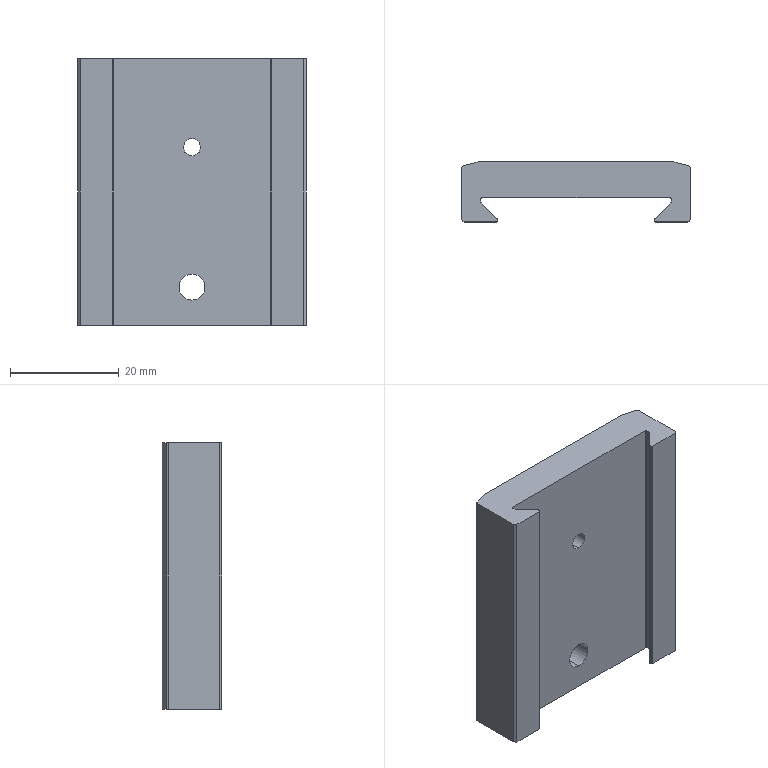Part | STEP file | 00382584_HALTER_SCHWALB._HMPL-..-.. | 1 solid | 39 faces | box 42 x 11 x 49 mm | volume 15212 mm3 | plane 18 | cylinder 16 | cone 5 | commonest cylinder face diameters 0.4 x10 0.8 x2 3.141 x2 4.773 x2